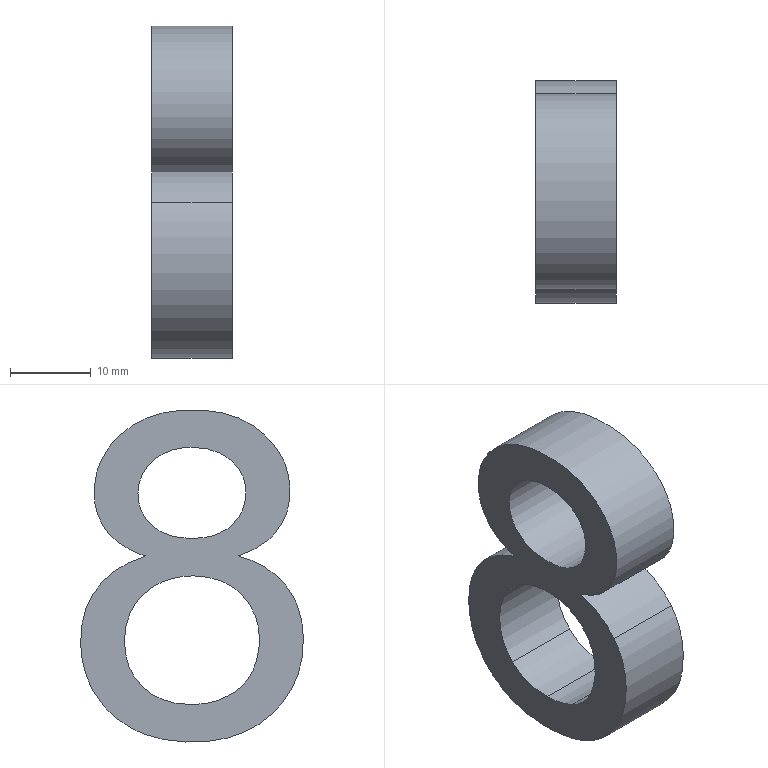Part | NX | features solid 2 | 1 solid | 12 faces | box 10 x 27.595 x 41.163 mm | volume 5547 mm3 | spline 10 | plane 2
STEP:
#1=CARTESIAN_POINT('',(2250.,-261.283,-555.936));
#2=VERTEX_POINT('',#1);
#3=CARTESIAN_POINT('',(2250.,-256.403,-554.268));
#4=VERTEX_POINT('',#3);
#5=CARTESIAN_POINT('',(2250.,-261.283,-555.936));
#6=CARTESIAN_POINT('',(2250.,-262.491,-557.021));
#7=CARTESIAN_POINT('',(2250.,-263.087,-558.306));
#8=CARTESIAN_POINT('',(2250.,-263.087,-561.488));
#9=CARTESIAN_POINT('',(2250.,-262.491,-562.864));
#10=CARTESIAN_POINT('',(2250.,-260.127,-565.013));
#11=CARTESIAN_POINT('',(2250.,-258.498,-565.556));
#12=CARTESIAN_POINT('',(2250.,-256.357,-565.556));
#13=CARTESIAN_POINT('',(2250.,-254.261,-565.556));
#14=CARTESIAN_POINT('',(2250.,-252.64,-565.021));
#15=CARTESIAN_POINT('',(2250.,-250.276,-562.903));
#16=CARTESIAN_POINT('',(2250.,-249.703,-561.579));
#17=CARTESIAN_POINT('',(2250.,-249.703,-558.428));
#18=CARTESIAN_POINT('',(2250.,-250.315,-557.067));
#19=CARTESIAN_POINT('',(2250.,-251.519,-555.962));
#20=CARTESIAN_POINT('',(2250.,-252.716,-554.864));
#21=CARTESIAN_POINT('',(2250.,-254.368,-554.298));
#22=CARTESIAN_POINT('',(2250.,-256.403,-554.268));
#23=B_SPLINE_CURVE_WITH_KNOTS('',3,(#5,#6,#7,#8,#9,#10,#11,#12,#13,#14,#15,#16,#17,#18,#19,#20,#21,#22),.UNSPECIFIED.,.F.,.F.,(4,2,2,3,2,2,3,4),(0.,0.1026,0.2247,0.3476,0.4748,0.6028,0.7308,0.8656),.UNSPECIFIED.);
#24=EDGE_CURVE('',#2,#4,#23,.T.);
#25=ORIENTED_EDGE('',*,*,#24,.F.);
#26=CARTESIAN_POINT('',(2260.,-261.283,-555.936));
#27=VERTEX_POINT('',#26);
#28=CARTESIAN_POINT('',(2260.,-261.283,-555.936));
#29=DIRECTION('',(-1.,0.,0.));
#30=VECTOR('',#29,1000.);
#31=LINE('',#28,#30);
#32=EDGE_CURVE('',#27,#2,#31,.T.);
#33=ORIENTED_EDGE('',*,*,#32,.F.);
#34=CARTESIAN_POINT('',(2260.,-256.403,-554.268));
#35=VERTEX_POINT('',#34);
#36=CARTESIAN_POINT('',(2260.,-261.283,-555.936));
#37=CARTESIAN_POINT('',(2260.,-262.491,-557.021));
#38=CARTESIAN_POINT('',(2260.,-263.087,-558.306));
#39=CARTESIAN_POINT('',(2260.,-263.087,-561.488));
#40=CARTESIAN_POINT('',(2260.,-262.491,-562.864));
#41=CARTESIAN_POINT('',(2260.,-260.127,-565.013));
#42=CARTESIAN_POINT('',(2260.,-258.498,-565.556));
#43=CARTESIAN_POINT('',(2260.,-256.357,-565.556));
#44=CARTESIAN_POINT('',(2260.,-254.261,-565.556));
#45=CARTESIAN_POINT('',(2260.,-252.64,-565.021));
#46=CARTESIAN_POINT('',(2260.,-250.276,-562.903));
#47=CARTESIAN_POINT('',(2260.,-249.703,-561.579));
#48=CARTESIAN_POINT('',(2260.,-249.703,-558.428));
#49=CARTESIAN_POINT('',(2260.,-250.315,-557.067));
#50=CARTESIAN_POINT('',(2260.,-251.519,-555.962));
#51=CARTESIAN_POINT('',(2260.,-252.716,-554.864));
#52=CARTESIAN_POINT('',(2260.,-254.368,-554.298));
#53=CARTESIAN_POINT('',(2260.,-256.403,-554.268));
#54=B_SPLINE_CURVE_WITH_KNOTS('',3,(#36,#37,#38,#39,#40,#41,#42,#43,#44,#45,#46,#47,#48,#49,#50,#51,#52,#53),.UNSPECIFIED.,.F.,.F.,(4,2,2,3,2,2,3,4),(0.,0.1026,0.2247,0.3476,0.4748,0.6028,0.7308,0.8656),.UNSPECIFIED.);
#55=EDGE_CURVE('',#27,#35,#54,.T.);
#56=ORIENTED_EDGE('',*,*,#55,.T.);
#57=CARTESIAN_POINT('',(2260.,-256.403,-554.268));
#58=DIRECTION('',(-1.,0.,0.));
#59=VECTOR('',#58,1000.);
#60=LINE('',#57,#59);
#61=EDGE_CURVE('',#4,#35,#60,.F.);
#62=ORIENTED_EDGE('',*,*,#61,.F.);
#63=EDGE_LOOP('',(#25,#33,#56,#62));
#64=FACE_BOUND('',#63,.T.);
#65=CARTESIAN_POINT('',(2260.,-261.283,-555.936));
#66=CARTESIAN_POINT('',(2250.,-261.283,-555.936));
#67=CARTESIAN_POINT('',(2260.,-261.919,-556.508));
#68=CARTESIAN_POINT('',(2250.,-261.919,-556.508));
#69=CARTESIAN_POINT('',(2260.,-262.862,-557.742));
#70=CARTESIAN_POINT('',(2250.,-262.862,-557.742));
#71=CARTESIAN_POINT('',(2260.,-263.216,-560.025));
#72=CARTESIAN_POINT('',(2250.,-263.216,-560.025));
#73=CARTESIAN_POINT('',(2260.,-262.775,-562.118));
#74=CARTESIAN_POINT('',(2250.,-262.775,-562.118));
#75=CARTESIAN_POINT('',(2260.,-261.656,-563.78));
#76=CARTESIAN_POINT('',(2250.,-261.656,-563.78));
#77=CARTESIAN_POINT('',(2260.,-259.878,-565.029));
#78=CARTESIAN_POINT('',(2250.,-259.878,-565.029));
#79=CARTESIAN_POINT('',(2260.,-258.006,-565.507));
#80=CARTESIAN_POINT('',(2250.,-258.006,-565.507));
#81=CARTESIAN_POINT('',(2260.,-256.133,-565.58));
#82=CARTESIAN_POINT('',(2250.,-256.133,-565.58));
#83=CARTESIAN_POINT('',(2260.,-254.468,-565.452));
#84=CARTESIAN_POINT('',(2250.,-254.468,-565.452));
#85=CARTESIAN_POINT('',(2260.,-252.698,-564.945));
#86=CARTESIAN_POINT('',(2250.,-252.698,-564.945));
#87=CARTESIAN_POINT('',(2260.,-251.039,-563.71));
#88=CARTESIAN_POINT('',(2250.,-251.039,-563.71));
#89=CARTESIAN_POINT('',(2260.,-250.002,-562.159));
#90=CARTESIAN_POINT('',(2250.,-250.002,-562.159));
#91=CARTESIAN_POINT('',(2260.,-249.605,-560.309));
#92=CARTESIAN_POINT('',(2250.,-249.605,-560.309));
#93=CARTESIAN_POINT('',(2260.,-249.832,-558.323));
#94=CARTESIAN_POINT('',(2250.,-249.832,-558.323));
#95=CARTESIAN_POINT('',(2260.,-250.724,-556.665));
#96=CARTESIAN_POINT('',(2250.,-250.724,-556.665));
#97=CARTESIAN_POINT('',(2260.,-252.714,-554.818));
#98=CARTESIAN_POINT('',(2250.,-252.714,-554.818));
#99=CARTESIAN_POINT('',(2260.,-254.769,-554.292));
#100=CARTESIAN_POINT('',(2250.,-254.769,-554.292));
#101=CARTESIAN_POINT('',(2260.,-256.403,-554.268));
#102=CARTESIAN_POINT('',(2250.,-256.403,-554.268));
#103=B_SPLINE_SURFACE_WITH_KNOTS('',3,1,((#65,#66),(#67,#68),(#69,#70),(#71,#72),(#73,#74),(#75,#76),(#77,#78),(#79,#80),(#81,#82),(#83,#84),(#85,#86),(#87,#88),(#89,#90),(#91,#92),(#93,#94),(#95,#96),(#97,#98),(#99,#100),(#101,#102)),.SURF_OF_LINEAR_EXTRUSION.,.F.,.F.,.F.,(4,1,1,1,1,1,1,1,1,1,1,1,1,1,1,1,4),(2,2),(0.,0.0541,0.1082,0.1623,0.2164,0.2705,0.3246,0.3516,0.3787,0.4328,0.4869,0.541,0.5951,0.6492,0.7033,0.7574,0.8656),(0.,1.),.UNSPECIFIED.);
#104=ADVANCED_FACE('',(#64),#103,.T.);
#105=CARTESIAN_POINT('',(2250.,-268.07,-571.451));
#106=VERTEX_POINT('',#105);
#107=CARTESIAN_POINT('',(2250.,-262.108,-567.728));
#108=VERTEX_POINT('',#107);
#109=CARTESIAN_POINT('',(2250.,-268.07,-571.451));
#110=CARTESIAN_POINT('',(2250.,-266.682,-569.671));
#111=CARTESIAN_POINT('',(2250.,-264.693,-568.402));
#112=CARTESIAN_POINT('',(2250.,-262.108,-567.728));
#113=B_SPLINE_CURVE_WITH_KNOTS('',3,(#109,#110,#111,#112),.UNSPECIFIED.,.F.,.F.,(4,4),(0.,0.05651),.PIECEWISE_BEZIER_KNOTS.);
#114=EDGE_CURVE('',#106,#108,#113,.T.);
#115=ORIENTED_EDGE('',*,*,#114,.F.);
#116=CARTESIAN_POINT('',(2260.,-268.07,-571.451));
#117=VERTEX_POINT('',#116);
#118=CARTESIAN_POINT('',(2260.,-268.07,-571.451));
#119=DIRECTION('',(-1.,0.,0.));
#120=VECTOR('',#119,1000.);
#121=LINE('',#118,#120);
#122=EDGE_CURVE('',#117,#106,#121,.T.);
#123=ORIENTED_EDGE('',*,*,#122,.F.);
#124=CARTESIAN_POINT('',(2260.,-262.108,-567.728));
#125=VERTEX_POINT('',#124);
#126=CARTESIAN_POINT('',(2260.,-268.07,-571.451));
#127=CARTESIAN_POINT('',(2260.,-266.682,-569.671));
#128=CARTESIAN_POINT('',(2260.,-264.693,-568.402));
#129=CARTESIAN_POINT('',(2260.,-262.108,-567.728));
#130=B_SPLINE_CURVE_WITH_KNOTS('',3,(#126,#127,#128,#129),.UNSPECIFIED.,.F.,.F.,(4,4),(0.,0.05651),.PIECEWISE_BEZIER_KNOTS.);
#131=EDGE_CURVE('',#117,#125,#130,.T.);
#132=ORIENTED_EDGE('',*,*,#131,.T.);
#133=CARTESIAN_POINT('',(2260.,-262.108,-567.728));
#134=DIRECTION('',(-1.,0.,0.));
#135=VECTOR('',#134,1000.);
#136=LINE('',#133,#135);
#137=EDGE_CURVE('',#125,#108,#136,.T.);
#138=ORIENTED_EDGE('',*,*,#137,.T.);
#139=EDGE_LOOP('',(#115,#123,#132,#138));
#140=FACE_BOUND('',#139,.T.);
#141=CARTESIAN_POINT('',(2260.,-268.07,-571.451));
#142=CARTESIAN_POINT('',(2250.,-268.07,-571.451));
#143=CARTESIAN_POINT('',(2260.,-266.682,-569.671));
#144=CARTESIAN_POINT('',(2250.,-266.682,-569.671));
#145=CARTESIAN_POINT('',(2260.,-264.693,-568.402));
#146=CARTESIAN_POINT('',(2250.,-264.693,-568.402));
#147=CARTESIAN_POINT('',(2260.,-262.108,-567.728));
#148=CARTESIAN_POINT('',(2250.,-262.108,-567.728));
#149=B_SPLINE_SURFACE_WITH_KNOTS('',3,1,((#141,#142),(#143,#144),(#145,#146),(#147,#148)),.SURF_OF_LINEAR_EXTRUSION.,.F.,.F.,.F.,(4,4),(2,2),(0.,0.05651),(0.,1.),.PIECEWISE_BEZIER_KNOTS.);
#150=ADVANCED_FACE('',(#140),#149,.T.);
#151=CARTESIAN_POINT('',(2250.,-250.605,-567.728));
#152=VERTEX_POINT('',#151);
#153=CARTESIAN_POINT('',(2250.,-262.108,-567.728));
#154=CARTESIAN_POINT('',(2250.,-264.265,-567.025));
#155=CARTESIAN_POINT('',(2250.,-265.886,-565.969));
#156=CARTESIAN_POINT('',(2250.,-267.977,-563.273));
#157=CARTESIAN_POINT('',(2250.,-268.533,-561.656));
#158=CARTESIAN_POINT('',(2250.,-268.533,-556.914));
#159=CARTESIAN_POINT('',(2250.,-267.431,-554.512));
#160=CARTESIAN_POINT('',(2250.,-263.056,-550.596));
#161=CARTESIAN_POINT('',(2250.,-260.12,-549.633));
#162=CARTESIAN_POINT('',(2250.,-252.823,-549.602));
#163=CARTESIAN_POINT('',(2250.,-249.871,-550.627));
#164=CARTESIAN_POINT('',(2250.,-245.382,-554.628));
#165=CARTESIAN_POINT('',(2250.,-244.273,-557.036));
#166=CARTESIAN_POINT('',(2250.,-244.273,-561.702));
#167=CARTESIAN_POINT('',(2250.,-244.793,-563.308));
#168=CARTESIAN_POINT('',(2250.,-246.888,-566.));
#169=CARTESIAN_POINT('',(2250.,-248.449,-567.025));
#170=CARTESIAN_POINT('',(2250.,-250.605,-567.728));
#171=B_SPLINE_CURVE_WITH_KNOTS('',3,(#153,#154,#155,#156,#157,#158,#159,#160,#161,#162,#163,#164,#165,#166,#167,#168,#169,#170),.UNSPECIFIED.,.F.,.F.,(4,2,2,2,2,2,2,2,4),(0.05651,0.1025,0.1475,0.2143,0.281,0.348,0.4148,0.4587,0.5037),.UNSPECIFIED.);
#172=EDGE_CURVE('',#108,#152,#171,.T.);
#173=ORIENTED_EDGE('',*,*,#172,.F.);
#174=ORIENTED_EDGE('',*,*,#137,.F.);
#175=CARTESIAN_POINT('',(2260.,-250.605,-567.728));
#176=VERTEX_POINT('',#175);
#177=CARTESIAN_POINT('',(2260.,-262.108,-567.728));
#178=CARTESIAN_POINT('',(2260.,-264.265,-567.025));
#179=CARTESIAN_POINT('',(2260.,-265.886,-565.969));
#180=CARTESIAN_POINT('',(2260.,-267.977,-563.273));
#181=CARTESIAN_POINT('',(2260.,-268.533,-561.656));
#182=CARTESIAN_POINT('',(2260.,-268.533,-556.914));
#183=CARTESIAN_POINT('',(2260.,-267.431,-554.512));
#184=CARTESIAN_POINT('',(2260.,-263.056,-550.596));
#185=CARTESIAN_POINT('',(2260.,-260.12,-549.633));
#186=CARTESIAN_POINT('',(2260.,-252.823,-549.602));
#187=CARTESIAN_POINT('',(2260.,-249.871,-550.627));
#188=CARTESIAN_POINT('',(2260.,-245.382,-554.628));
#189=CARTESIAN_POINT('',(2260.,-244.273,-557.036));
#190=CARTESIAN_POINT('',(2260.,-244.273,-561.702));
#191=CARTESIAN_POINT('',(2260.,-244.793,-563.308));
#192=CARTESIAN_POINT('',(2260.,-246.888,-566.));
#193=CARTESIAN_POINT('',(2260.,-248.449,-567.025));
#194=CARTESIAN_POINT('',(2260.,-250.605,-567.728));
#195=B_SPLINE_CURVE_WITH_KNOTS('',3,(#177,#178,#179,#180,#181,#182,#183,#184,#185,#186,#187,#188,#189,#190,#191,#192,#193,#194),.UNSPECIFIED.,.F.,.F.,(4,2,2,2,2,2,2,2,4),(0.05651,0.1025,0.1475,0.2143,0.281,0.348,0.4148,0.4587,0.5037),.UNSPECIFIED.);
#196=EDGE_CURVE('',#125,#176,#195,.T.);
#197=ORIENTED_EDGE('',*,*,#196,.T.);
#198=CARTESIAN_POINT('',(2260.,-250.605,-567.728));
#199=DIRECTION('',(-1.,0.,0.));
#200=VECTOR('',#199,1000.);
#201=LINE('',#198,#200);
#202=EDGE_CURVE('',#176,#152,#201,.T.);
#203=ORIENTED_EDGE('',*,*,#202,.T.);
#204=EDGE_LOOP('',(#173,#174,#197,#203));
#205=FACE_BOUND('',#204,.T.);
#206=CARTESIAN_POINT('',(2260.,-262.108,-567.728));
#207=CARTESIAN_POINT('',(2250.,-262.108,-567.728));
#208=CARTESIAN_POINT('',(2260.,-264.731,-566.873));
#209=CARTESIAN_POINT('',(2250.,-264.731,-566.873));
#210=CARTESIAN_POINT('',(2260.,-267.434,-564.8));
#211=CARTESIAN_POINT('',(2250.,-267.434,-564.8));
#212=CARTESIAN_POINT('',(2260.,-268.541,-561.267));
#213=CARTESIAN_POINT('',(2250.,-268.541,-561.267));
#214=CARTESIAN_POINT('',(2260.,-268.547,-558.873));
#215=CARTESIAN_POINT('',(2250.,-268.547,-558.873));
#216=CARTESIAN_POINT('',(2260.,-268.165,-556.653));
#217=CARTESIAN_POINT('',(2250.,-268.165,-556.653));
#218=CARTESIAN_POINT('',(2260.,-266.978,-554.174));
#219=CARTESIAN_POINT('',(2250.,-266.978,-554.174));
#220=CARTESIAN_POINT('',(2260.,-264.349,-551.574));
#221=CARTESIAN_POINT('',(2250.,-264.349,-551.574));
#222=CARTESIAN_POINT('',(2260.,-261.494,-550.264));
#223=CARTESIAN_POINT('',(2250.,-261.494,-550.264));
#224=CARTESIAN_POINT('',(2260.,-258.845,-549.728));
#225=CARTESIAN_POINT('',(2250.,-258.845,-549.728));
#226=CARTESIAN_POINT('',(2260.,-256.632,-549.576));
#227=CARTESIAN_POINT('',(2250.,-256.632,-549.576));
#228=CARTESIAN_POINT('',(2260.,-254.379,-549.682));
#229=CARTESIAN_POINT('',(2250.,-254.379,-549.682));
#230=CARTESIAN_POINT('',(2260.,-251.696,-550.186));
#231=CARTESIAN_POINT('',(2250.,-251.696,-550.186));
#232=CARTESIAN_POINT('',(2260.,-248.779,-551.472));
#233=CARTESIAN_POINT('',(2250.,-248.779,-551.472));
#234=CARTESIAN_POINT('',(2260.,-246.005,-554.071));
#235=CARTESIAN_POINT('',(2250.,-246.005,-554.071));
#236=CARTESIAN_POINT('',(2260.,-244.728,-556.534));
#237=CARTESIAN_POINT('',(2250.,-244.728,-556.534));
#238=CARTESIAN_POINT('',(2260.,-244.284,-558.719));
#239=CARTESIAN_POINT('',(2250.,-244.284,-558.719));
#240=CARTESIAN_POINT('',(2260.,-244.225,-561.096));
#241=CARTESIAN_POINT('',(2250.,-244.225,-561.096));
#242=CARTESIAN_POINT('',(2260.,-245.238,-564.753));
#243=CARTESIAN_POINT('',(2250.,-245.238,-564.753));
#244=CARTESIAN_POINT('',(2260.,-247.924,-566.854));
#245=CARTESIAN_POINT('',(2250.,-247.924,-566.854));
#246=CARTESIAN_POINT('',(2260.,-250.605,-567.728));
#247=CARTESIAN_POINT('',(2250.,-250.605,-567.728));
#248=B_SPLINE_SURFACE_WITH_KNOTS('',3,1,((#206,#207),(#208,#209),(#210,#211),(#212,#213),(#214,#215),(#216,#217),(#218,#219),(#220,#221),(#222,#223),(#224,#225),(#226,#227),(#228,#229),(#230,#231),(#232,#233),(#234,#235),(#236,#237),(#238,#239),(#240,#241),(#242,#243),(#244,#245),(#246,#247)),.SURF_OF_LINEAR_EXTRUSION.,.F.,.F.,.F.,(4,1,1,1,1,1,1,1,1,1,1,1,1,1,1,1,1,1,4),(2,2),(0.05651,0.1124,0.1404,0.1543,0.1683,0.1962,0.2242,0.2521,0.2661,0.2801,0.2941,0.308,0.336,0.3639,0.3919,0.4059,0.4198,0.4478,0.5037),(0.,1.),.UNSPECIFIED.);
#249=ADVANCED_FACE('',(#205),#248,.T.);
#250=CARTESIAN_POINT('',(2250.,-250.284,-583.912));
#251=VERTEX_POINT('',#250);
#252=CARTESIAN_POINT('',(2250.,-256.54,-570.191));
#253=VERTEX_POINT('',#252);
#254=CARTESIAN_POINT('',(2250.,-250.284,-583.912));
#255=CARTESIAN_POINT('',(2250.,-248.77,-582.459));
#256=CARTESIAN_POINT('',(2250.,-248.036,-580.562));
#257=CARTESIAN_POINT('',(2250.,-248.036,-575.958));
#258=CARTESIAN_POINT('',(2250.,-248.8,-574.031));
#259=CARTESIAN_POINT('',(2250.,-251.898,-570.994));
#260=CARTESIAN_POINT('',(2250.,-253.971,-570.222));
#261=CARTESIAN_POINT('',(2250.,-256.54,-570.191));
#262=B_SPLINE_CURVE_WITH_KNOTS('',3,(#254,#255,#256,#257,#258,#259,#260,#261),.UNSPECIFIED.,.F.,.F.,(4,2,2,4),(0.5085,0.6312,0.7532,0.8733),.UNSPECIFIED.);
#263=EDGE_CURVE('',#251,#253,#262,.T.);
#264=ORIENTED_EDGE('',*,*,#263,.F.);
#265=CARTESIAN_POINT('',(2260.,-250.284,-583.912));
#266=VERTEX_POINT('',#265);
#267=CARTESIAN_POINT('',(2260.,-250.284,-583.912));
#268=DIRECTION('',(-1.,0.,0.));
#269=VECTOR('',#268,1000.);
#270=LINE('',#267,#269);
#271=EDGE_CURVE('',#266,#251,#270,.T.);
#272=ORIENTED_EDGE('',*,*,#271,.F.);
#273=CARTESIAN_POINT('',(2260.,-256.54,-570.191));
#274=VERTEX_POINT('',#273);
#275=CARTESIAN_POINT('',(2260.,-250.284,-583.912));
#276=CARTESIAN_POINT('',(2260.,-248.77,-582.459));
#277=CARTESIAN_POINT('',(2260.,-248.036,-580.562));
#278=CARTESIAN_POINT('',(2260.,-248.036,-575.958));
#279=CARTESIAN_POINT('',(2260.,-248.8,-574.031));
#280=CARTESIAN_POINT('',(2260.,-251.898,-570.994));
#281=CARTESIAN_POINT('',(2260.,-253.971,-570.222));
#282=CARTESIAN_POINT('',(2260.,-256.54,-570.191));
#283=B_SPLINE_CURVE_WITH_KNOTS('',3,(#275,#276,#277,#278,#279,#280,#281,#282),.UNSPECIFIED.,.F.,.F.,(4,2,2,4),(0.5085,0.6312,0.7532,0.8733),.UNSPECIFIED.);
#284=EDGE_CURVE('',#266,#274,#283,.T.);
#285=ORIENTED_EDGE('',*,*,#284,.T.);
#286=CARTESIAN_POINT('',(2260.,-256.54,-570.191));
#287=DIRECTION('',(-1.,0.,0.));
#288=VECTOR('',#287,1000.);
#289=LINE('',#286,#288);
#290=EDGE_CURVE('',#274,#253,#289,.T.);
#291=ORIENTED_EDGE('',*,*,#290,.T.);
#292=EDGE_LOOP('',(#264,#272,#285,#291));
#293=FACE_BOUND('',#292,.T.);
#294=CARTESIAN_POINT('',(2260.,-250.284,-583.912));
#295=CARTESIAN_POINT('',(2250.,-250.284,-583.912));
#296=CARTESIAN_POINT('',(2260.,-249.159,-582.832));
#297=CARTESIAN_POINT('',(2250.,-249.159,-582.832));
#298=CARTESIAN_POINT('',(2260.,-248.12,-580.887));
#299=CARTESIAN_POINT('',(2250.,-248.12,-580.887));
#300=CARTESIAN_POINT('',(2260.,-247.959,-577.431));
#301=CARTESIAN_POINT('',(2250.,-247.959,-577.431));
#302=CARTESIAN_POINT('',(2260.,-248.479,-575.096));
#303=CARTESIAN_POINT('',(2250.,-248.479,-575.096));
#304=CARTESIAN_POINT('',(2260.,-249.655,-573.095));
#305=CARTESIAN_POINT('',(2250.,-249.655,-573.095));
#306=CARTESIAN_POINT('',(2260.,-252.104,-570.873));
#307=CARTESIAN_POINT('',(2250.,-252.104,-570.873));
#308=CARTESIAN_POINT('',(2260.,-254.589,-570.214));
#309=CARTESIAN_POINT('',(2250.,-254.589,-570.214));
#310=CARTESIAN_POINT('',(2260.,-256.54,-570.191));
#311=CARTESIAN_POINT('',(2250.,-256.54,-570.191));
#312=B_SPLINE_SURFACE_WITH_KNOTS('',3,1,((#294,#295),(#296,#297),(#298,#299),(#300,#301),(#302,#303),(#304,#305),(#306,#307),(#308,#309),(#310,#311)),.SURF_OF_LINEAR_EXTRUSION.,.F.,.F.,.F.,(4,1,1,1,1,1,4),(2,2),(0.5085,0.5997,0.6453,0.6909,0.7365,0.7821,0.8733),(0.,1.),.UNSPECIFIED.);
#313=ADVANCED_FACE('',(#293),#312,.T.);
#314=CARTESIAN_POINT('',(2250.,-262.52,-572.485));
#315=VERTEX_POINT('',#314);
#316=CARTESIAN_POINT('',(2250.,-256.54,-570.191));
#317=CARTESIAN_POINT('',(2250.,-259.049,-570.222));
#318=CARTESIAN_POINT('',(2250.,-261.022,-570.971));
#319=CARTESIAN_POINT('',(2250.,-262.52,-572.485));
#320=B_SPLINE_CURVE_WITH_KNOTS('',3,(#316,#317,#318,#319),.UNSPECIFIED.,.F.,.F.,(4,4),(0.8733,1.),.PIECEWISE_BEZIER_KNOTS.);
#321=EDGE_CURVE('',#253,#315,#320,.T.);
#322=ORIENTED_EDGE('',*,*,#321,.F.);
#323=ORIENTED_EDGE('',*,*,#290,.F.);
#324=CARTESIAN_POINT('',(2260.,-262.52,-572.485));
#325=VERTEX_POINT('',#324);
#326=CARTESIAN_POINT('',(2260.,-256.54,-570.191));
#327=CARTESIAN_POINT('',(2260.,-259.049,-570.222));
#328=CARTESIAN_POINT('',(2260.,-261.022,-570.971));
#329=CARTESIAN_POINT('',(2260.,-262.52,-572.485));
#330=B_SPLINE_CURVE_WITH_KNOTS('',3,(#326,#327,#328,#329),.UNSPECIFIED.,.F.,.F.,(4,4),(0.8733,1.),.PIECEWISE_BEZIER_KNOTS.);
#331=EDGE_CURVE('',#274,#325,#330,.T.);
#332=ORIENTED_EDGE('',*,*,#331,.T.);
#333=CARTESIAN_POINT('',(2260.,-262.52,-572.485));
#334=DIRECTION('',(-1.,0.,0.));
#335=VECTOR('',#334,1000.);
#336=LINE('',#333,#335);
#337=EDGE_CURVE('',#325,#315,#336,.T.);
#338=ORIENTED_EDGE('',*,*,#337,.T.);
#339=EDGE_LOOP('',(#322,#323,#332,#338));
#340=FACE_BOUND('',#339,.T.);
#341=CARTESIAN_POINT('',(2260.,-256.54,-570.191));
#342=CARTESIAN_POINT('',(2250.,-256.54,-570.191));
#343=CARTESIAN_POINT('',(2260.,-259.049,-570.222));
#344=CARTESIAN_POINT('',(2250.,-259.049,-570.222));
#345=CARTESIAN_POINT('',(2260.,-261.022,-570.971));
#346=CARTESIAN_POINT('',(2250.,-261.022,-570.971));
#347=CARTESIAN_POINT('',(2260.,-262.52,-572.485));
#348=CARTESIAN_POINT('',(2250.,-262.52,-572.485));
#349=B_SPLINE_SURFACE_WITH_KNOTS('',3,1,((#341,#342),(#343,#344),(#345,#346),(#347,#348)),.SURF_OF_LINEAR_EXTRUSION.,.F.,.F.,.F.,(4,4),(2,2),(0.8733,1.),(0.,1.),.PIECEWISE_BEZIER_KNOTS.);
#350=ADVANCED_FACE('',(#340),#349,.T.);
#351=CARTESIAN_POINT('',(2250.,-260.823,-585.075));
#352=VERTEX_POINT('',#351);
#353=CARTESIAN_POINT('',(2250.,-262.52,-572.485));
#354=CARTESIAN_POINT('',(2250.,-264.005,-573.985));
#355=CARTESIAN_POINT('',(2250.,-264.77,-575.851));
#356=CARTESIAN_POINT('',(2250.,-264.77,-579.491));
#357=CARTESIAN_POINT('',(2250.,-264.449,-580.837));
#358=CARTESIAN_POINT('',(2250.,-263.226,-583.408));
#359=CARTESIAN_POINT('',(2250.,-262.231,-584.402));
#360=CARTESIAN_POINT('',(2250.,-260.823,-585.075));
#361=B_SPLINE_CURVE_WITH_KNOTS('',3,(#353,#354,#355,#356,#357,#358,#359,#360),.UNSPECIFIED.,.F.,.F.,(4,2,2,4),(0.,0.1255,0.2046,0.2876),.UNSPECIFIED.);
#362=EDGE_CURVE('',#315,#352,#361,.T.);
#363=ORIENTED_EDGE('',*,*,#362,.F.);
#364=ORIENTED_EDGE('',*,*,#337,.F.);
#365=CARTESIAN_POINT('',(2260.,-260.823,-585.075));
#366=VERTEX_POINT('',#365);
#367=CARTESIAN_POINT('',(2260.,-262.52,-572.485));
#368=CARTESIAN_POINT('',(2260.,-264.005,-573.985));
#369=CARTESIAN_POINT('',(2260.,-264.77,-575.851));
#370=CARTESIAN_POINT('',(2260.,-264.77,-579.491));
#371=CARTESIAN_POINT('',(2260.,-264.449,-580.837));
#372=CARTESIAN_POINT('',(2260.,-263.226,-583.408));
#373=CARTESIAN_POINT('',(2260.,-262.231,-584.402));
#374=CARTESIAN_POINT('',(2260.,-260.823,-585.075));
#375=B_SPLINE_CURVE_WITH_KNOTS('',3,(#367,#368,#369,#370,#371,#372,#373,#374),.UNSPECIFIED.,.F.,.F.,(4,2,2,4),(0.,0.1255,0.2046,0.2876),.UNSPECIFIED.);
#376=EDGE_CURVE('',#325,#366,#375,.T.);
#377=ORIENTED_EDGE('',*,*,#376,.T.);
#378=CARTESIAN_POINT('',(2260.,-260.823,-585.075));
#379=DIRECTION('',(-1.,0.,0.));
#380=VECTOR('',#379,1000.);
#381=LINE('',#378,#380);
#382=EDGE_CURVE('',#366,#352,#381,.T.);
#383=ORIENTED_EDGE('',*,*,#382,.T.);
#384=EDGE_LOOP('',(#363,#364,#377,#383));
#385=FACE_BOUND('',#384,.T.);
#386=CARTESIAN_POINT('',(2260.,-262.52,-572.485));
#387=CARTESIAN_POINT('',(2250.,-262.52,-572.485));
#388=CARTESIAN_POINT('',(2260.,-263.371,-573.344));
#389=CARTESIAN_POINT('',(2250.,-263.371,-573.344));
#390=CARTESIAN_POINT('',(2260.,-264.292,-574.816));
#391=CARTESIAN_POINT('',(2250.,-264.292,-574.816));
#392=CARTESIAN_POINT('',(2260.,-264.787,-577.128));
#393=CARTESIAN_POINT('',(2250.,-264.787,-577.128));
#394=CARTESIAN_POINT('',(2260.,-264.785,-579.07));
#395=CARTESIAN_POINT('',(2250.,-264.785,-579.07));
#396=CARTESIAN_POINT('',(2260.,-264.389,-580.891));
#397=CARTESIAN_POINT('',(2250.,-264.389,-580.891));
#398=CARTESIAN_POINT('',(2260.,-263.405,-583.251));
#399=CARTESIAN_POINT('',(2250.,-263.405,-583.251));
#400=CARTESIAN_POINT('',(2260.,-262.043,-584.491));
#401=CARTESIAN_POINT('',(2250.,-262.043,-584.491));
#402=CARTESIAN_POINT('',(2260.,-260.823,-585.075));
#403=CARTESIAN_POINT('',(2250.,-260.823,-585.075));
#404=B_SPLINE_SURFACE_WITH_KNOTS('',3,1,((#386,#387),(#388,#389),(#390,#391),(#392,#393),(#394,#395),(#396,#397),(#398,#399),(#400,#401),(#402,#403)),.SURF_OF_LINEAR_EXTRUSION.,.F.,.F.,.F.,(4,1,1,1,1,1,4),(2,2),(0.,0.07189,0.1078,0.1438,0.1797,0.2157,0.2876),(0.,1.),.UNSPECIFIED.);
#405=ADVANCED_FACE('',(#385),#404,.T.);
#406=CARTESIAN_POINT('',(2250.,-256.372,-586.115));
#407=VERTEX_POINT('',#406);
#408=CARTESIAN_POINT('',(2250.,-260.823,-585.075));
#409=CARTESIAN_POINT('',(2250.,-259.416,-585.809));
#410=CARTESIAN_POINT('',(2250.,-257.917,-586.145));
#411=CARTESIAN_POINT('',(2250.,-256.372,-586.115));
#412=B_SPLINE_CURVE_WITH_KNOTS('',3,(#408,#409,#410,#411),.UNSPECIFIED.,.F.,.F.,(4,4),(0.2876,0.378),.PIECEWISE_BEZIER_KNOTS.);
#413=EDGE_CURVE('',#352,#407,#412,.T.);
#414=ORIENTED_EDGE('',*,*,#413,.F.);
#415=ORIENTED_EDGE('',*,*,#382,.F.);
#416=CARTESIAN_POINT('',(2260.,-256.372,-586.115));
#417=VERTEX_POINT('',#416);
#418=CARTESIAN_POINT('',(2260.,-260.823,-585.075));
#419=CARTESIAN_POINT('',(2260.,-259.416,-585.809));
#420=CARTESIAN_POINT('',(2260.,-257.917,-586.145));
#421=CARTESIAN_POINT('',(2260.,-256.372,-586.115));
#422=B_SPLINE_CURVE_WITH_KNOTS('',3,(#418,#419,#420,#421),.UNSPECIFIED.,.F.,.F.,(4,4),(0.2876,0.378),.PIECEWISE_BEZIER_KNOTS.);
#423=EDGE_CURVE('',#366,#417,#422,.T.);
#424=ORIENTED_EDGE('',*,*,#423,.T.);
#425=CARTESIAN_POINT('',(2260.,-256.372,-586.115));
#426=DIRECTION('',(-1.,0.,0.));
#427=VECTOR('',#426,1000.);
#428=LINE('',#425,#427);
#429=EDGE_CURVE('',#417,#407,#428,.T.);
#430=ORIENTED_EDGE('',*,*,#429,.T.);
#431=EDGE_LOOP('',(#414,#415,#424,#430));
#432=FACE_BOUND('',#431,.T.);
#433=CARTESIAN_POINT('',(2260.,-260.823,-585.075));
#434=CARTESIAN_POINT('',(2250.,-260.823,-585.075));
#435=CARTESIAN_POINT('',(2260.,-259.416,-585.809));
#436=CARTESIAN_POINT('',(2250.,-259.416,-585.809));
#437=CARTESIAN_POINT('',(2260.,-257.917,-586.145));
#438=CARTESIAN_POINT('',(2250.,-257.917,-586.145));
#439=CARTESIAN_POINT('',(2260.,-256.372,-586.115));
#440=CARTESIAN_POINT('',(2250.,-256.372,-586.115));
#441=B_SPLINE_SURFACE_WITH_KNOTS('',3,1,((#433,#434),(#435,#436),(#437,#438),(#439,#440)),.SURF_OF_LINEAR_EXTRUSION.,.F.,.F.,.F.,(4,4),(2,2),(0.2876,0.378),(0.,1.),.PIECEWISE_BEZIER_KNOTS.);
#442=ADVANCED_FACE('',(#432),#441,.T.);
#443=CARTESIAN_POINT('',(2250.,-250.605,-567.728));
#444=CARTESIAN_POINT('',(2250.,-247.99,-568.57));
#445=CARTESIAN_POINT('',(2250.,-246.001,-569.901));
#446=CARTESIAN_POINT('',(2250.,-243.264,-573.561));
#447=CARTESIAN_POINT('',(2250.,-242.605,-575.774));
#448=CARTESIAN_POINT('',(2250.,-242.605,-581.847));
#449=CARTESIAN_POINT('',(2250.,-243.86,-584.83));
#450=CARTESIAN_POINT('',(2250.,-248.923,-589.617));
#451=CARTESIAN_POINT('',(2250.,-252.273,-590.78));
#452=CARTESIAN_POINT('',(2250.,-260.533,-590.78));
#453=CARTESIAN_POINT('',(2250.,-263.883,-589.618));
#454=CARTESIAN_POINT('',(2250.,-268.915,-584.798));
#455=CARTESIAN_POINT('',(2250.,-270.2,-581.801));
#456=CARTESIAN_POINT('',(2250.,-270.2,-575.514));
#457=CARTESIAN_POINT('',(2250.,-269.496,-573.281));
#458=CARTESIAN_POINT('',(2250.,-268.07,-571.451));
#459=B_SPLINE_CURVE_WITH_KNOTS('',3,(#443,#444,#445,#446,#447,#448,#449,#450,#451,#452,#453,#454,#455,#456,#457,#458),.UNSPECIFIED.,.F.,.F.,(4,2,2,2,2,2,2,4),(0.5037,0.5606,0.6182,0.6991,0.7805,0.862,0.9419,1.),.UNSPECIFIED.);
#460=EDGE_CURVE('',#152,#106,#459,.T.);
#461=ORIENTED_EDGE('',*,*,#460,.F.);
#462=ORIENTED_EDGE('',*,*,#202,.F.);
#463=CARTESIAN_POINT('',(2260.,-250.605,-567.728));
#464=CARTESIAN_POINT('',(2260.,-247.99,-568.57));
#465=CARTESIAN_POINT('',(2260.,-246.001,-569.901));
#466=CARTESIAN_POINT('',(2260.,-243.264,-573.561));
#467=CARTESIAN_POINT('',(2260.,-242.605,-575.774));
#468=CARTESIAN_POINT('',(2260.,-242.605,-581.847));
#469=CARTESIAN_POINT('',(2260.,-243.86,-584.83));
#470=CARTESIAN_POINT('',(2260.,-248.923,-589.617));
#471=CARTESIAN_POINT('',(2260.,-252.273,-590.78));
#472=CARTESIAN_POINT('',(2260.,-260.533,-590.78));
#473=CARTESIAN_POINT('',(2260.,-263.883,-589.618));
#474=CARTESIAN_POINT('',(2260.,-268.915,-584.798));
#475=CARTESIAN_POINT('',(2260.,-270.2,-581.801));
#476=CARTESIAN_POINT('',(2260.,-270.2,-575.514));
#477=CARTESIAN_POINT('',(2260.,-269.496,-573.281));
#478=CARTESIAN_POINT('',(2260.,-268.07,-571.451));
#479=B_SPLINE_CURVE_WITH_KNOTS('',3,(#463,#464,#465,#466,#467,#468,#469,#470,#471,#472,#473,#474,#475,#476,#477,#478),.UNSPECIFIED.,.F.,.F.,(4,2,2,2,2,2,2,4),(0.5037,0.5606,0.6182,0.6991,0.7805,0.862,0.9419,1.),.UNSPECIFIED.);
#480=EDGE_CURVE('',#176,#117,#479,.T.);
#481=ORIENTED_EDGE('',*,*,#480,.T.);
#482=ORIENTED_EDGE('',*,*,#122,.T.);
#483=EDGE_LOOP('',(#461,#462,#481,#482));
#484=FACE_BOUND('',#483,.T.);
#485=CARTESIAN_POINT('',(2260.,-250.605,-567.728));
#486=CARTESIAN_POINT('',(2250.,-250.605,-567.728));
#487=CARTESIAN_POINT('',(2260.,-247.755,-568.645));
#488=CARTESIAN_POINT('',(2250.,-247.755,-568.645));
#489=CARTESIAN_POINT('',(2260.,-244.563,-570.953));
#490=CARTESIAN_POINT('',(2250.,-244.563,-570.953));
#491=CARTESIAN_POINT('',(2260.,-242.917,-574.949));
#492=CARTESIAN_POINT('',(2250.,-242.917,-574.949));
#493=CARTESIAN_POINT('',(2260.,-242.578,-577.506));
#494=CARTESIAN_POINT('',(2250.,-242.578,-577.506));
#495=CARTESIAN_POINT('',(2260.,-242.624,-580.246));
#496=CARTESIAN_POINT('',(2250.,-242.624,-580.246));
#497=CARTESIAN_POINT('',(2260.,-243.368,-583.288));
#498=CARTESIAN_POINT('',(2250.,-243.368,-583.288));
#499=CARTESIAN_POINT('',(2260.,-245.383,-586.466));
#500=CARTESIAN_POINT('',(2250.,-245.383,-586.466));
#501=CARTESIAN_POINT('',(2260.,-248.482,-589.068));
#502=CARTESIAN_POINT('',(2250.,-248.482,-589.068));
#503=CARTESIAN_POINT('',(2260.,-251.596,-590.27));
#504=CARTESIAN_POINT('',(2250.,-251.596,-590.27));
#505=CARTESIAN_POINT('',(2260.,-254.42,-590.731));
#506=CARTESIAN_POINT('',(2250.,-254.42,-590.731));
#507=CARTESIAN_POINT('',(2260.,-257.559,-590.849));
#508=CARTESIAN_POINT('',(2250.,-257.559,-590.849));
#509=CARTESIAN_POINT('',(2260.,-261.211,-590.36));
#510=CARTESIAN_POINT('',(2250.,-261.211,-590.36));
#511=CARTESIAN_POINT('',(2260.,-264.826,-588.74));
#512=CARTESIAN_POINT('',(2250.,-264.826,-588.74));
#513=CARTESIAN_POINT('',(2260.,-267.805,-585.964));
#514=CARTESIAN_POINT('',(2250.,-267.805,-585.964));
#515=CARTESIAN_POINT('',(2260.,-269.656,-582.671));
#516=CARTESIAN_POINT('',(2250.,-269.656,-582.671));
#517=CARTESIAN_POINT('',(2260.,-270.263,-579.421));
#518=CARTESIAN_POINT('',(2250.,-270.263,-579.421));
#519=CARTESIAN_POINT('',(2260.,-270.167,-576.589));
#520=CARTESIAN_POINT('',(2250.,-270.167,-576.589));
#521=CARTESIAN_POINT('',(2260.,-269.664,-574.072));
#522=CARTESIAN_POINT('',(2250.,-269.664,-574.072));
#523=CARTESIAN_POINT('',(2260.,-268.831,-572.428));
#524=CARTESIAN_POINT('',(2250.,-268.831,-572.428));
#525=CARTESIAN_POINT('',(2260.,-268.07,-571.451));
#526=CARTESIAN_POINT('',(2250.,-268.07,-571.451));
#527=B_SPLINE_SURFACE_WITH_KNOTS('',3,1,((#485,#486),(#487,#488),(#489,#490),(#491,#492),(#493,#494),(#495,#496),(#497,#498),(#499,#500),(#501,#502),(#503,#504),(#505,#506),(#507,#508),(#509,#510),(#511,#512),(#513,#514),(#515,#516),(#517,#518),(#519,#520),(#521,#522),(#523,#524),(#525,#526)),.SURF_OF_LINEAR_EXTRUSION.,.F.,.F.,.F.,(4,1,1,1,1,1,1,1,1,1,1,1,1,1,1,1,1,1,4),(2,2),(0.5037,0.5657,0.5967,0.6122,0.6278,0.6588,0.6898,0.7208,0.7518,0.7673,0.7829,0.8139,0.8449,0.8759,0.9069,0.938,0.9535,0.969,1.),(0.,1.),.UNSPECIFIED.);
#528=ADVANCED_FACE('',(#484),#527,.T.);
#529=CARTESIAN_POINT('',(2250.,-256.372,-586.115));
#530=CARTESIAN_POINT('',(2250.,-253.818,-586.145));
#531=CARTESIAN_POINT('',(2250.,-251.768,-585.411));
#532=CARTESIAN_POINT('',(2250.,-250.284,-583.912));
#533=B_SPLINE_CURVE_WITH_KNOTS('',3,(#529,#530,#531,#532),.UNSPECIFIED.,.F.,.F.,(4,4),(0.378,0.5085),.PIECEWISE_BEZIER_KNOTS.);
#534=EDGE_CURVE('',#407,#251,#533,.T.);
#535=ORIENTED_EDGE('',*,*,#534,.F.);
#536=ORIENTED_EDGE('',*,*,#429,.F.);
#537=CARTESIAN_POINT('',(2260.,-256.372,-586.115));
#538=CARTESIAN_POINT('',(2260.,-253.818,-586.145));
#539=CARTESIAN_POINT('',(2260.,-251.768,-585.411));
#540=CARTESIAN_POINT('',(2260.,-250.284,-583.912));
#541=B_SPLINE_CURVE_WITH_KNOTS('',3,(#537,#538,#539,#540),.UNSPECIFIED.,.F.,.F.,(4,4),(0.378,0.5085),.PIECEWISE_BEZIER_KNOTS.);
#542=EDGE_CURVE('',#417,#266,#541,.T.);
#543=ORIENTED_EDGE('',*,*,#542,.T.);
#544=ORIENTED_EDGE('',*,*,#271,.T.);
#545=EDGE_LOOP('',(#535,#536,#543,#544));
#546=FACE_BOUND('',#545,.T.);
#547=CARTESIAN_POINT('',(2260.,-256.372,-586.115));
#548=CARTESIAN_POINT('',(2250.,-256.372,-586.115));
#549=CARTESIAN_POINT('',(2260.,-253.818,-586.145));
#550=CARTESIAN_POINT('',(2250.,-253.818,-586.145));
#551=CARTESIAN_POINT('',(2260.,-251.768,-585.411));
#552=CARTESIAN_POINT('',(2250.,-251.768,-585.411));
#553=CARTESIAN_POINT('',(2260.,-250.284,-583.912));
#554=CARTESIAN_POINT('',(2250.,-250.284,-583.912));
#555=B_SPLINE_SURFACE_WITH_KNOTS('',3,1,((#547,#548),(#549,#550),(#551,#552),(#553,#554)),.SURF_OF_LINEAR_EXTRUSION.,.F.,.F.,.F.,(4,4),(2,2),(0.378,0.5085),(0.,1.),.PIECEWISE_BEZIER_KNOTS.);
#556=ADVANCED_FACE('',(#546),#555,.T.);
#557=CARTESIAN_POINT('',(2250.,-256.403,-554.268));
#558=CARTESIAN_POINT('',(2250.,-258.468,-554.298));
#559=CARTESIAN_POINT('',(2250.,-260.089,-554.864));
#560=CARTESIAN_POINT('',(2250.,-261.283,-555.936));
#561=B_SPLINE_CURVE_WITH_KNOTS('',3,(#557,#558,#559,#560),.UNSPECIFIED.,.F.,.F.,(4,4),(0.8656,1.),.PIECEWISE_BEZIER_KNOTS.);
#562=EDGE_CURVE('',#4,#2,#561,.T.);
#563=ORIENTED_EDGE('',*,*,#562,.F.);
#564=ORIENTED_EDGE('',*,*,#61,.T.);
#565=CARTESIAN_POINT('',(2260.,-256.403,-554.268));
#566=CARTESIAN_POINT('',(2260.,-258.468,-554.298));
#567=CARTESIAN_POINT('',(2260.,-260.089,-554.864));
#568=CARTESIAN_POINT('',(2260.,-261.283,-555.936));
#569=B_SPLINE_CURVE_WITH_KNOTS('',3,(#565,#566,#567,#568),.UNSPECIFIED.,.F.,.F.,(4,4),(0.8656,1.),.PIECEWISE_BEZIER_KNOTS.);
#570=EDGE_CURVE('',#35,#27,#569,.T.);
#571=ORIENTED_EDGE('',*,*,#570,.T.);
#572=ORIENTED_EDGE('',*,*,#32,.T.);
#573=EDGE_LOOP('',(#563,#564,#571,#572));
#574=FACE_BOUND('',#573,.T.);
#575=CARTESIAN_POINT('',(2260.,-256.403,-554.268));
#576=CARTESIAN_POINT('',(2250.,-256.403,-554.268));
#577=CARTESIAN_POINT('',(2260.,-258.468,-554.298));
#578=CARTESIAN_POINT('',(2250.,-258.468,-554.298));
#579=CARTESIAN_POINT('',(2260.,-260.089,-554.864));
#580=CARTESIAN_POINT('',(2250.,-260.089,-554.864));
#581=CARTESIAN_POINT('',(2260.,-261.283,-555.936));
#582=CARTESIAN_POINT('',(2250.,-261.283,-555.936));
#583=B_SPLINE_SURFACE_WITH_KNOTS('',3,1,((#575,#576),(#577,#578),(#579,#580),(#581,#582)),.SURF_OF_LINEAR_EXTRUSION.,.F.,.F.,.F.,(4,4),(2,2),(0.8656,1.),(0.,1.),.PIECEWISE_BEZIER_KNOTS.);
#584=ADVANCED_FACE('',(#574),#583,.T.);
#585=ORIENTED_EDGE('',*,*,#284,.F.);
#586=ORIENTED_EDGE('',*,*,#542,.F.);
#587=ORIENTED_EDGE('',*,*,#423,.F.);
#588=ORIENTED_EDGE('',*,*,#376,.F.);
#589=ORIENTED_EDGE('',*,*,#331,.F.);
#590=EDGE_LOOP('',(#585,#586,#587,#588,#589));
#591=FACE_BOUND('',#590,.T.);
#592=ORIENTED_EDGE('',*,*,#131,.F.);
#593=ORIENTED_EDGE('',*,*,#480,.F.);
#594=ORIENTED_EDGE('',*,*,#196,.F.);
#595=EDGE_LOOP('',(#592,#593,#594));
#596=FACE_BOUND('',#595,.T.);
#597=ORIENTED_EDGE('',*,*,#55,.F.);
#598=ORIENTED_EDGE('',*,*,#570,.F.);
#599=EDGE_LOOP('',(#597,#598));
#600=FACE_BOUND('',#599,.T.);
#601=CARTESIAN_POINT('',(2260.,-265.538,-569.175));
#602=DIRECTION('',(1.,0.,0.));
#603=DIRECTION('',(0.,1.,0.));
#604=AXIS2_PLACEMENT_3D('',#601,#602,#603);
#605=PLANE('',#604);
#606=ADVANCED_FACE('',(#591,#596,#600),#605,.T.);
#607=ORIENTED_EDGE('',*,*,#263,.T.);
#608=ORIENTED_EDGE('',*,*,#321,.T.);
#609=ORIENTED_EDGE('',*,*,#362,.T.);
#610=ORIENTED_EDGE('',*,*,#413,.T.);
#611=ORIENTED_EDGE('',*,*,#534,.T.);
#612=EDGE_LOOP('',(#607,#608,#609,#610,#611));
#613=FACE_BOUND('',#612,.T.);
#614=ORIENTED_EDGE('',*,*,#114,.T.);
#615=ORIENTED_EDGE('',*,*,#172,.T.);
#616=ORIENTED_EDGE('',*,*,#460,.T.);
#617=EDGE_LOOP('',(#614,#615,#616));
#618=FACE_BOUND('',#617,.T.);
#619=ORIENTED_EDGE('',*,*,#24,.T.);
#620=ORIENTED_EDGE('',*,*,#562,.T.);
#621=EDGE_LOOP('',(#619,#620));
#622=FACE_BOUND('',#621,.T.);
#623=CARTESIAN_POINT('',(2250.,-265.538,-569.175));
#624=DIRECTION('',(1.,0.,0.));
#625=DIRECTION('',(0.,1.,0.));
#626=AXIS2_PLACEMENT_3D('',#623,#624,#625);
#627=PLANE('',#626);
#628=ADVANCED_FACE('',(#613,#618,#622),#627,.F.);
#629=CLOSED_SHELL('',(#104,#150,#249,#313,#350,#405,#442,#528,#556,#584,#606,#628));
#630=MANIFOLD_SOLID_BREP('',#629);
#631=(LENGTH_UNIT()NAMED_UNIT(*)SI_UNIT(.MILLI.,.METRE.));
#632=UNCERTAINTY_MEASURE_WITH_UNIT(LENGTH_MEASURE(0.0508),#631,'','');
#633=(NAMED_UNIT(*)PLANE_ANGLE_UNIT()SI_UNIT($,.RADIAN.));
#634=(NAMED_UNIT(*)SI_UNIT($,.STERADIAN.)SOLID_ANGLE_UNIT());
#635=(GEOMETRIC_REPRESENTATION_CONTEXT(3)GLOBAL_UNCERTAINTY_ASSIGNED_CONTEXT((#632))GLOBAL_UNIT_ASSIGNED_CONTEXT((#631,#633,#634))REPRESENTATION_CONTEXT('',''));
#636=ADVANCED_BREP_SHAPE_REPRESENTATION('',(#630),#635);